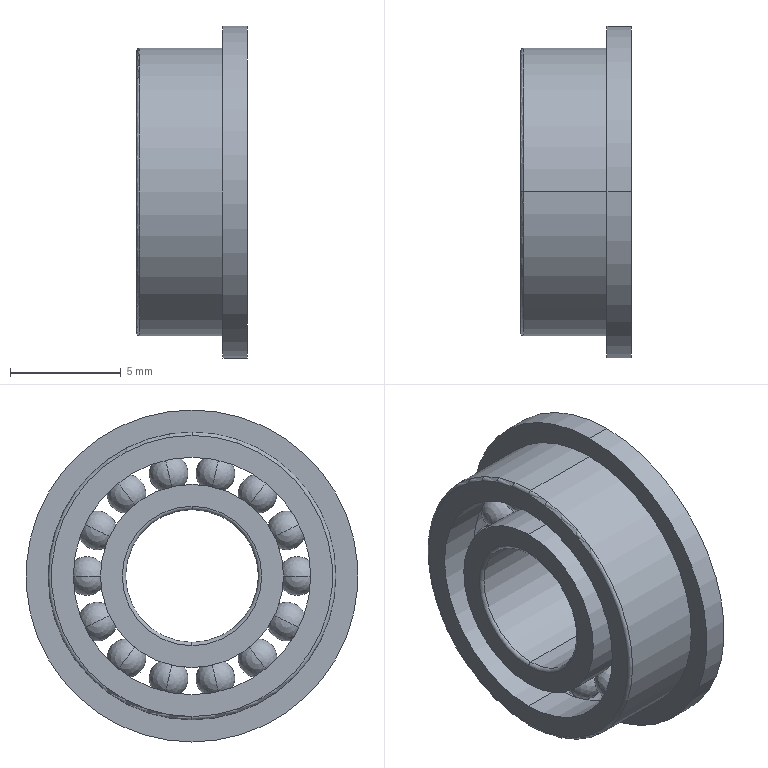Part | SolidWorks | features BaseBody 16 | 16 solids | 87 faces | box 5 x 15 x 15 mm | volume 413.271 mm3 | sphere 56 | cylinder 14 | torus 12 | plane 5 | commonest cylinder face diameters 8.275 x4 10.725 x4 6 x2 13 x2 15 x2